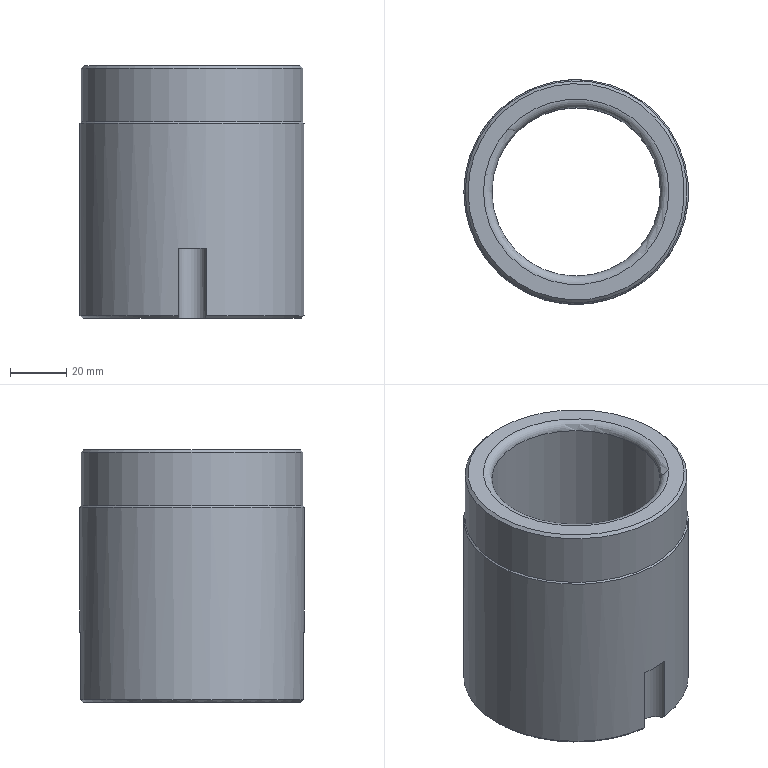Part | NX | features solid 2 | 1 solid | 16 faces | box 80 x 80 x 90 mm | volume 190213 mm3 | cone 5 | cylinder 5 | plane 4 | torus 2 | commonest cylinder face diameters 10 x2 60 x1 79 x1 80 x1
STEP:
#1=CARTESIAN_POINT('',(1209.99,-155.312,-129.));
#2=VERTEX_POINT('',#1);
#3=CARTESIAN_POINT('',(1209.828,-156.3,-130.));
#4=VERTEX_POINT('',#3);
#5=CARTESIAN_POINT('',(1209.99,-155.312,-129.));
#6=CARTESIAN_POINT('',(1209.969,-155.646,-129.334));
#7=CARTESIAN_POINT('',(1209.915,-155.976,-129.667));
#8=CARTESIAN_POINT('',(1209.828,-156.3,-130.));
#9=B_SPLINE_CURVE_WITH_KNOTS('',3,(#5,#6,#7,#8),.UNSPECIFIED.,.F.,.F.,(4,4),(0.000000282,0.001415),.UNSPECIFIED.);
#10=EDGE_CURVE('',#2,#4,#9,.T.);
#11=ORIENTED_EDGE('',*,*,#10,.F.);
#12=CARTESIAN_POINT('',(1209.99,-234.688,-129.));
#13=VERTEX_POINT('',#12);
#14=CARTESIAN_POINT('',(1205.,-195.,-129.));
#15=DIRECTION('',(0.,0.,-1.));
#16=DIRECTION('',(1.,0.,0.));
#17=AXIS2_PLACEMENT_3D('',#14,#15,#16);
#18=CIRCLE('',#17,40.);
#19=EDGE_CURVE('',#13,#2,#18,.F.);
#20=ORIENTED_EDGE('',*,*,#19,.F.);
#21=CARTESIAN_POINT('',(1209.828,-233.7,-130.));
#22=VERTEX_POINT('',#21);
#23=CARTESIAN_POINT('',(1209.828,-233.7,-130.));
#24=CARTESIAN_POINT('',(1209.915,-234.024,-129.667));
#25=CARTESIAN_POINT('',(1209.969,-234.354,-129.334));
#26=CARTESIAN_POINT('',(1209.99,-234.688,-129.));
#27=B_SPLINE_CURVE_WITH_KNOTS('',3,(#23,#24,#25,#26),.UNSPECIFIED.,.F.,.F.,(4,4),(0.000000284,0.001415),.UNSPECIFIED.);
#28=EDGE_CURVE('',#22,#13,#27,.T.);
#29=ORIENTED_EDGE('',*,*,#28,.F.);
#30=CARTESIAN_POINT('',(1205.,-195.,-130.));
#31=DIRECTION('',(0.,0.,-1.));
#32=DIRECTION('',(1.,0.,0.));
#33=AXIS2_PLACEMENT_3D('',#30,#31,#32);
#34=CIRCLE('',#33,39.);
#35=EDGE_CURVE('',#4,#22,#34,.T.);
#36=ORIENTED_EDGE('',*,*,#35,.F.);
#37=EDGE_LOOP('',(#11,#20,#29,#36));
#38=FACE_BOUND('',#37,.T.);
#39=CARTESIAN_POINT('',(1205.,-195.,-129.));
#40=DIRECTION('',(0.,0.,1.));
#41=DIRECTION('',(-1.,0.,0.));
#42=AXIS2_PLACEMENT_3D('',#39,#40,#41);
#43=CONICAL_SURFACE('',#42,40.,0.7854);
#44=ADVANCED_FACE('',(#38),#43,.T.);
#45=CARTESIAN_POINT('',(1200.172,-156.3,-130.));
#46=VERTEX_POINT('',#45);
#47=CARTESIAN_POINT('',(1205.,-155.,-130.));
#48=DIRECTION('',(0.,0.,1.));
#49=DIRECTION('',(-1.,0.,0.));
#50=AXIS2_PLACEMENT_3D('',#47,#48,#49);
#51=CIRCLE('',#50,5.);
#52=EDGE_CURVE('',#46,#4,#51,.T.);
#53=ORIENTED_EDGE('',*,*,#52,.T.);
#54=ORIENTED_EDGE('',*,*,#35,.T.);
#55=CARTESIAN_POINT('',(1200.172,-233.7,-130.));
#56=VERTEX_POINT('',#55);
#57=CARTESIAN_POINT('',(1205.,-235.,-130.));
#58=DIRECTION('',(0.,0.,1.));
#59=DIRECTION('',(-1.,0.,0.));
#60=AXIS2_PLACEMENT_3D('',#57,#58,#59);
#61=CIRCLE('',#60,5.);
#62=EDGE_CURVE('',#22,#56,#61,.T.);
#63=ORIENTED_EDGE('',*,*,#62,.T.);
#64=CARTESIAN_POINT('',(1205.,-195.,-130.));
#65=DIRECTION('',(0.,0.,-1.));
#66=DIRECTION('',(1.,0.,0.));
#67=AXIS2_PLACEMENT_3D('',#64,#65,#66);
#68=CIRCLE('',#67,39.);
#69=EDGE_CURVE('',#56,#46,#68,.T.);
#70=ORIENTED_EDGE('',*,*,#69,.T.);
#71=EDGE_LOOP('',(#53,#54,#63,#70));
#72=FACE_BOUND('',#71,.T.);
#73=CARTESIAN_POINT('',(1172.321,-195.,-130.));
#74=VERTEX_POINT('',#73);
#75=CARTESIAN_POINT('',(1205.,-195.,-130.));
#76=DIRECTION('',(0.,0.,1.));
#77=DIRECTION('',(-1.,0.,0.));
#78=AXIS2_PLACEMENT_3D('',#75,#76,#77);
#79=CIRCLE('',#78,32.679);
#80=EDGE_CURVE('',#74,#74,#79,.T.);
#81=ORIENTED_EDGE('',*,*,#80,.T.);
#82=EDGE_LOOP('',(#81));
#83=FACE_BOUND('',#82,.T.);
#84=CARTESIAN_POINT('',(1205.,-195.,-130.));
#85=DIRECTION('',(0.,0.,-1.));
#86=DIRECTION('',(1.,0.,0.));
#87=AXIS2_PLACEMENT_3D('',#84,#85,#86);
#88=PLANE('',#87);
#89=ADVANCED_FACE('',(#72,#83),#88,.T.);
#90=CARTESIAN_POINT('',(1200.01,-155.312,-129.));
#91=VERTEX_POINT('',#90);
#92=CARTESIAN_POINT('',(1200.01,-155.312,-105.));
#93=VERTEX_POINT('',#92);
#94=CARTESIAN_POINT('',(1200.01,-155.312,-117.5));
#95=DIRECTION('',(0.,0.,1.));
#96=VECTOR('',#95,1000.);
#97=LINE('',#94,#96);
#98=EDGE_CURVE('',#91,#93,#97,.T.);
#99=ORIENTED_EDGE('',*,*,#98,.F.);
#100=CARTESIAN_POINT('',(1200.01,-234.688,-129.));
#101=VERTEX_POINT('',#100);
#102=CARTESIAN_POINT('',(1205.,-195.,-129.));
#103=DIRECTION('',(0.,0.,-1.));
#104=DIRECTION('',(1.,0.,0.));
#105=AXIS2_PLACEMENT_3D('',#102,#103,#104);
#106=CIRCLE('',#105,40.);
#107=EDGE_CURVE('',#91,#101,#106,.F.);
#108=ORIENTED_EDGE('',*,*,#107,.T.);
#109=CARTESIAN_POINT('',(1200.01,-234.688,-105.));
#110=VERTEX_POINT('',#109);
#111=CARTESIAN_POINT('',(1200.01,-234.688,-117.5));
#112=DIRECTION('',(0.,0.,1.));
#113=VECTOR('',#112,1000.);
#114=LINE('',#111,#113);
#115=EDGE_CURVE('',#110,#101,#114,.F.);
#116=ORIENTED_EDGE('',*,*,#115,.F.);
#117=CARTESIAN_POINT('',(1209.99,-234.688,-105.));
#118=VERTEX_POINT('',#117);
#119=CARTESIAN_POINT('',(1205.,-195.,-105.));
#120=DIRECTION('',(0.,0.,1.));
#121=DIRECTION('',(-1.,0.,0.));
#122=AXIS2_PLACEMENT_3D('',#119,#120,#121);
#123=CIRCLE('',#122,40.);
#124=EDGE_CURVE('',#118,#110,#123,.F.);
#125=ORIENTED_EDGE('',*,*,#124,.F.);
#126=CARTESIAN_POINT('',(1209.99,-234.688,-117.5));
#127=DIRECTION('',(0.,0.,1.));
#128=VECTOR('',#127,1000.);
#129=LINE('',#126,#128);
#130=EDGE_CURVE('',#13,#118,#129,.T.);
#131=ORIENTED_EDGE('',*,*,#130,.F.);
#132=ORIENTED_EDGE('',*,*,#19,.T.);
#133=CARTESIAN_POINT('',(1209.99,-155.312,-105.));
#134=VERTEX_POINT('',#133);
#135=CARTESIAN_POINT('',(1209.99,-155.312,-117.5));
#136=DIRECTION('',(0.,0.,1.));
#137=VECTOR('',#136,1000.);
#138=LINE('',#135,#137);
#139=EDGE_CURVE('',#134,#2,#138,.F.);
#140=ORIENTED_EDGE('',*,*,#139,.F.);
#141=CARTESIAN_POINT('',(1205.,-195.,-105.));
#142=DIRECTION('',(0.,0.,1.));
#143=DIRECTION('',(-1.,0.,0.));
#144=AXIS2_PLACEMENT_3D('',#141,#142,#143);
#145=CIRCLE('',#144,40.);
#146=EDGE_CURVE('',#93,#134,#145,.F.);
#147=ORIENTED_EDGE('',*,*,#146,.F.);
#148=EDGE_LOOP('',(#99,#108,#116,#125,#131,#132,#140,#147));
#149=FACE_BOUND('',#148,.T.);
#150=CARTESIAN_POINT('',(1165.,-195.,-60.5));
#151=VERTEX_POINT('',#150);
#152=CARTESIAN_POINT('',(1205.,-195.,-60.5));
#153=DIRECTION('',(0.,0.,1.));
#154=DIRECTION('',(-1.,0.,0.));
#155=AXIS2_PLACEMENT_3D('',#152,#153,#154);
#156=CIRCLE('',#155,40.);
#157=EDGE_CURVE('',#151,#151,#156,.F.);
#158=ORIENTED_EDGE('',*,*,#157,.T.);
#159=EDGE_LOOP('',(#158));
#160=FACE_BOUND('',#159,.T.);
#161=CARTESIAN_POINT('',(1205.,-195.,-130.));
#162=DIRECTION('',(0.,0.,1.));
#163=DIRECTION('',(-1.,0.,0.));
#164=AXIS2_PLACEMENT_3D('',#161,#162,#163);
#165=CYLINDRICAL_SURFACE('',#164,40.);
#166=ADVANCED_FACE('',(#149,#160),#165,.T.);
#167=CARTESIAN_POINT('',(1166.5,-195.,-40.));
#168=VERTEX_POINT('',#167);
#169=CARTESIAN_POINT('',(1205.,-195.,-40.));
#170=DIRECTION('',(0.,0.,1.));
#171=DIRECTION('',(-1.,0.,0.));
#172=AXIS2_PLACEMENT_3D('',#169,#170,#171);
#173=CIRCLE('',#172,38.5);
#174=EDGE_CURVE('',#168,#168,#173,.T.);
#175=ORIENTED_EDGE('',*,*,#174,.T.);
#176=EDGE_LOOP('',(#175));
#177=FACE_BOUND('',#176,.T.);
#178=CARTESIAN_POINT('',(1172.,-195.,-40.));
#179=VERTEX_POINT('',#178);
#180=CARTESIAN_POINT('',(1205.,-195.,-40.));
#181=DIRECTION('',(0.,0.,1.));
#182=DIRECTION('',(-1.,0.,0.));
#183=AXIS2_PLACEMENT_3D('',#180,#181,#182);
#184=CIRCLE('',#183,33.);
#185=EDGE_CURVE('',#179,#179,#184,.F.);
#186=ORIENTED_EDGE('',*,*,#185,.T.);
#187=EDGE_LOOP('',(#186));
#188=FACE_BOUND('',#187,.T.);
#189=CARTESIAN_POINT('',(1205.,-195.,-40.));
#190=DIRECTION('',(0.,0.,1.));
#191=DIRECTION('',(-1.,0.,0.));
#192=AXIS2_PLACEMENT_3D('',#189,#190,#191);
#193=PLANE('',#192);
#194=ADVANCED_FACE('',(#177,#188),#193,.T.);
#195=CARTESIAN_POINT('',(1165.5,-195.,-41.));
#196=VERTEX_POINT('',#195);
#197=CARTESIAN_POINT('',(1205.,-195.,-41.));
#198=DIRECTION('',(0.,0.,1.));
#199=DIRECTION('',(-1.,0.,0.));
#200=AXIS2_PLACEMENT_3D('',#197,#198,#199);
#201=CIRCLE('',#200,39.5);
#202=EDGE_CURVE('',#196,#196,#201,.F.);
#203=ORIENTED_EDGE('',*,*,#202,.T.);
#204=EDGE_LOOP('',(#203));
#205=FACE_BOUND('',#204,.T.);
#206=CARTESIAN_POINT('',(1165.5,-195.,-60.));
#207=VERTEX_POINT('',#206);
#208=CARTESIAN_POINT('',(1205.,-195.,-60.));
#209=DIRECTION('',(0.,0.,1.));
#210=DIRECTION('',(-1.,0.,0.));
#211=AXIS2_PLACEMENT_3D('',#208,#209,#210);
#212=CIRCLE('',#211,39.5);
#213=EDGE_CURVE('',#207,#207,#212,.T.);
#214=ORIENTED_EDGE('',*,*,#213,.T.);
#215=EDGE_LOOP('',(#214));
#216=FACE_BOUND('',#215,.T.);
#217=CARTESIAN_POINT('',(1205.,-195.,-40.));
#218=DIRECTION('',(0.,0.,-1.));
#219=DIRECTION('',(1.,0.,0.));
#220=AXIS2_PLACEMENT_3D('',#217,#218,#219);
#221=CYLINDRICAL_SURFACE('',#220,39.5);
#222=ADVANCED_FACE('',(#205,#216),#221,.T.);
#223=CARTESIAN_POINT('',(1174.319,-195.,-122.543));
#224=VERTEX_POINT('',#223);
#225=CARTESIAN_POINT('',(1205.,-195.,-122.543));
#226=DIRECTION('',(0.,0.,1.));
#227=DIRECTION('',(-1.,0.,0.));
#228=AXIS2_PLACEMENT_3D('',#225,#226,#227);
#229=CIRCLE('',#228,30.681);
#230=EDGE_CURVE('',#224,#224,#229,.T.);
#231=ORIENTED_EDGE('',*,*,#230,.T.);
#232=EDGE_LOOP('',(#231));
#233=FACE_BOUND('',#232,.T.);
#234=ORIENTED_EDGE('',*,*,#80,.F.);
#235=EDGE_LOOP('',(#234));
#236=FACE_BOUND('',#235,.T.);
#237=CARTESIAN_POINT('',(1205.,-195.,-120.));
#238=DIRECTION('',(0.,0.,-1.));
#239=DIRECTION('',(1.,0.,0.));
#240=AXIS2_PLACEMENT_3D('',#237,#238,#239);
#241=CONICAL_SURFACE('',#240,30.,0.2618);
#242=ADVANCED_FACE('',(#233,#236),#241,.F.);
#243=CARTESIAN_POINT('',(1175.,-195.,-43.));
#244=VERTEX_POINT('',#243);
#245=CARTESIAN_POINT('',(1205.,-195.,-43.));
#246=DIRECTION('',(0.,0.,1.));
#247=DIRECTION('',(-1.,0.,0.));
#248=AXIS2_PLACEMENT_3D('',#245,#246,#247);
#249=CIRCLE('',#248,30.);
#250=EDGE_CURVE('',#244,#244,#249,.T.);
#251=ORIENTED_EDGE('',*,*,#250,.T.);
#252=EDGE_LOOP('',(#251));
#253=FACE_BOUND('',#252,.T.);
#254=CARTESIAN_POINT('',(1235.,-195.,-117.367));
#255=VERTEX_POINT('',#254);
#256=CARTESIAN_POINT('',(1205.,-195.,-117.367));
#257=DIRECTION('',(0.,0.,-1.));
#258=DIRECTION('',(1.,0.,0.));
#259=AXIS2_PLACEMENT_3D('',#256,#257,#258);
#260=CIRCLE('',#259,30.);
#261=EDGE_CURVE('',#255,#255,#260,.T.);
#262=ORIENTED_EDGE('',*,*,#261,.T.);
#263=EDGE_LOOP('',(#262));
#264=FACE_BOUND('',#263,.T.);
#265=CARTESIAN_POINT('',(1205.,-195.,-130.));
#266=DIRECTION('',(0.,0.,1.));
#267=DIRECTION('',(-1.,0.,0.));
#268=AXIS2_PLACEMENT_3D('',#265,#266,#267);
#269=CYLINDRICAL_SURFACE('',#268,30.);
#270=ADVANCED_FACE('',(#253,#264),#269,.F.);
#271=ORIENTED_EDGE('',*,*,#261,.F.);
#272=EDGE_LOOP('',(#271));
#273=FACE_BOUND('',#272,.T.);
#274=ORIENTED_EDGE('',*,*,#230,.F.);
#275=EDGE_LOOP('',(#274));
#276=FACE_BOUND('',#275,.T.);
#277=CARTESIAN_POINT('',(1205.,-195.,-117.367));
#278=DIRECTION('',(0.,0.,-1.));
#279=DIRECTION('',(1.,0.,0.));
#280=AXIS2_PLACEMENT_3D('',#277,#278,#279);
#281=TOROIDAL_SURFACE('',#280,50.,20.);
#282=ADVANCED_FACE('',(#273,#276),#281,.T.);
#283=ORIENTED_EDGE('',*,*,#250,.F.);
#284=EDGE_LOOP('',(#283));
#285=FACE_BOUND('',#284,.T.);
#286=ORIENTED_EDGE('',*,*,#185,.F.);
#287=EDGE_LOOP('',(#286));
#288=FACE_BOUND('',#287,.T.);
#289=CARTESIAN_POINT('',(1205.,-195.,-43.));
#290=DIRECTION('',(0.,0.,1.));
#291=DIRECTION('',(-1.,0.,0.));
#292=AXIS2_PLACEMENT_3D('',#289,#290,#291);
#293=TOROIDAL_SURFACE('',#292,33.,3.);
#294=ADVANCED_FACE('',(#285,#288),#293,.T.);
#295=ORIENTED_EDGE('',*,*,#174,.F.);
#296=EDGE_LOOP('',(#295));
#297=FACE_BOUND('',#296,.T.);
#298=ORIENTED_EDGE('',*,*,#202,.F.);
#299=EDGE_LOOP('',(#298));
#300=FACE_BOUND('',#299,.T.);
#301=CARTESIAN_POINT('',(1205.,-195.,-41.));
#302=DIRECTION('',(0.,0.,-1.));
#303=DIRECTION('',(1.,0.,0.));
#304=AXIS2_PLACEMENT_3D('',#301,#302,#303);
#305=CONICAL_SURFACE('',#304,39.5,0.7854);
#306=ADVANCED_FACE('',(#297,#300),#305,.T.);
#307=CARTESIAN_POINT('',(1200.172,-156.3,-130.));
#308=CARTESIAN_POINT('',(1200.085,-155.976,-129.667));
#309=CARTESIAN_POINT('',(1200.031,-155.646,-129.334));
#310=CARTESIAN_POINT('',(1200.01,-155.312,-129.));
#311=B_SPLINE_CURVE_WITH_KNOTS('',3,(#307,#308,#309,#310),.UNSPECIFIED.,.F.,.F.,(4,4),(0.000000284,0.001415),.UNSPECIFIED.);
#312=EDGE_CURVE('',#46,#91,#311,.T.);
#313=ORIENTED_EDGE('',*,*,#312,.F.);
#314=ORIENTED_EDGE('',*,*,#69,.F.);
#315=CARTESIAN_POINT('',(1200.01,-234.688,-129.));
#316=CARTESIAN_POINT('',(1200.031,-234.354,-129.334));
#317=CARTESIAN_POINT('',(1200.085,-234.024,-129.667));
#318=CARTESIAN_POINT('',(1200.172,-233.7,-130.));
#319=B_SPLINE_CURVE_WITH_KNOTS('',3,(#315,#316,#317,#318),.UNSPECIFIED.,.F.,.F.,(4,4),(0.000000282,0.001415),.UNSPECIFIED.);
#320=EDGE_CURVE('',#101,#56,#319,.T.);
#321=ORIENTED_EDGE('',*,*,#320,.F.);
#322=ORIENTED_EDGE('',*,*,#107,.F.);
#323=EDGE_LOOP('',(#313,#314,#321,#322));
#324=FACE_BOUND('',#323,.T.);
#325=CARTESIAN_POINT('',(1205.,-195.,-129.));
#326=DIRECTION('',(0.,0.,1.));
#327=DIRECTION('',(-1.,0.,0.));
#328=AXIS2_PLACEMENT_3D('',#325,#326,#327);
#329=CONICAL_SURFACE('',#328,40.,0.7854);
#330=ADVANCED_FACE('',(#324),#329,.T.);
#331=ORIENTED_EDGE('',*,*,#213,.F.);
#332=EDGE_LOOP('',(#331));
#333=FACE_BOUND('',#332,.T.);
#334=ORIENTED_EDGE('',*,*,#157,.F.);
#335=EDGE_LOOP('',(#334));
#336=FACE_BOUND('',#335,.T.);
#337=CARTESIAN_POINT('',(1205.,-195.,-60.5));
#338=DIRECTION('',(0.,0.,-1.));
#339=DIRECTION('',(1.,0.,0.));
#340=AXIS2_PLACEMENT_3D('',#337,#338,#339);
#341=CONICAL_SURFACE('',#340,40.,0.7854);
#342=ADVANCED_FACE('',(#333,#336),#341,.T.);
#343=ORIENTED_EDGE('',*,*,#124,.T.);
#344=CARTESIAN_POINT('',(1205.,-235.,-105.));
#345=DIRECTION('',(0.,0.,-1.));
#346=DIRECTION('',(1.,0.,0.));
#347=AXIS2_PLACEMENT_3D('',#344,#345,#346);
#348=CIRCLE('',#347,5.);
#349=EDGE_CURVE('',#110,#118,#348,.T.);
#350=ORIENTED_EDGE('',*,*,#349,.T.);
#351=EDGE_LOOP('',(#343,#350));
#352=FACE_BOUND('',#351,.T.);
#353=CARTESIAN_POINT('',(1205.,-235.,-105.));
#354=DIRECTION('',(0.,0.,1.));
#355=DIRECTION('',(-1.,0.,0.));
#356=AXIS2_PLACEMENT_3D('',#353,#354,#355);
#357=PLANE('',#356);
#358=ADVANCED_FACE('',(#352),#357,.F.);
#359=ORIENTED_EDGE('',*,*,#115,.T.);
#360=ORIENTED_EDGE('',*,*,#320,.T.);
#361=ORIENTED_EDGE('',*,*,#62,.F.);
#362=ORIENTED_EDGE('',*,*,#28,.T.);
#363=ORIENTED_EDGE('',*,*,#130,.T.);
#364=ORIENTED_EDGE('',*,*,#349,.F.);
#365=EDGE_LOOP('',(#359,#360,#361,#362,#363,#364));
#366=FACE_BOUND('',#365,.T.);
#367=CARTESIAN_POINT('',(1205.,-235.,-130.));
#368=DIRECTION('',(0.,0.,1.));
#369=DIRECTION('',(-1.,0.,0.));
#370=AXIS2_PLACEMENT_3D('',#367,#368,#369);
#371=CYLINDRICAL_SURFACE('',#370,5.);
#372=ADVANCED_FACE('',(#366),#371,.F.);
#373=ORIENTED_EDGE('',*,*,#146,.T.);
#374=CARTESIAN_POINT('',(1205.,-155.,-105.));
#375=DIRECTION('',(0.,0.,-1.));
#376=DIRECTION('',(1.,0.,0.));
#377=AXIS2_PLACEMENT_3D('',#374,#375,#376);
#378=CIRCLE('',#377,5.);
#379=EDGE_CURVE('',#134,#93,#378,.T.);
#380=ORIENTED_EDGE('',*,*,#379,.T.);
#381=EDGE_LOOP('',(#373,#380));
#382=FACE_BOUND('',#381,.T.);
#383=CARTESIAN_POINT('',(1205.,-155.,-105.));
#384=DIRECTION('',(0.,0.,1.));
#385=DIRECTION('',(-1.,0.,0.));
#386=AXIS2_PLACEMENT_3D('',#383,#384,#385);
#387=PLANE('',#386);
#388=ADVANCED_FACE('',(#382),#387,.F.);
#389=ORIENTED_EDGE('',*,*,#139,.T.);
#390=ORIENTED_EDGE('',*,*,#10,.T.);
#391=ORIENTED_EDGE('',*,*,#52,.F.);
#392=ORIENTED_EDGE('',*,*,#312,.T.);
#393=ORIENTED_EDGE('',*,*,#98,.T.);
#394=ORIENTED_EDGE('',*,*,#379,.F.);
#395=EDGE_LOOP('',(#389,#390,#391,#392,#393,#394));
#396=FACE_BOUND('',#395,.T.);
#397=CARTESIAN_POINT('',(1205.,-155.,-130.));
#398=DIRECTION('',(0.,0.,1.));
#399=DIRECTION('',(-1.,0.,0.));
#400=AXIS2_PLACEMENT_3D('',#397,#398,#399);
#401=CYLINDRICAL_SURFACE('',#400,5.);
#402=ADVANCED_FACE('',(#396),#401,.F.);
#403=CLOSED_SHELL('',(#44,#89,#166,#194,#222,#242,#270,#282,#294,#306,#330,#342,#358,#372,#388,#402));
#404=MANIFOLD_SOLID_BREP('',#403);
#405=(LENGTH_UNIT()NAMED_UNIT(*)SI_UNIT(.MILLI.,.METRE.));
#406=UNCERTAINTY_MEASURE_WITH_UNIT(LENGTH_MEASURE(0.0508),#405,'','');
#407=(NAMED_UNIT(*)PLANE_ANGLE_UNIT()SI_UNIT($,.RADIAN.));
#408=(NAMED_UNIT(*)SI_UNIT($,.STERADIAN.)SOLID_ANGLE_UNIT());
#409=(GEOMETRIC_REPRESENTATION_CONTEXT(3)GLOBAL_UNCERTAINTY_ASSIGNED_CONTEXT((#406))GLOBAL_UNIT_ASSIGNED_CONTEXT((#405,#407,#408))REPRESENTATION_CONTEXT('',''));
#410=ADVANCED_BREP_SHAPE_REPRESENTATION('',(#404),#409);